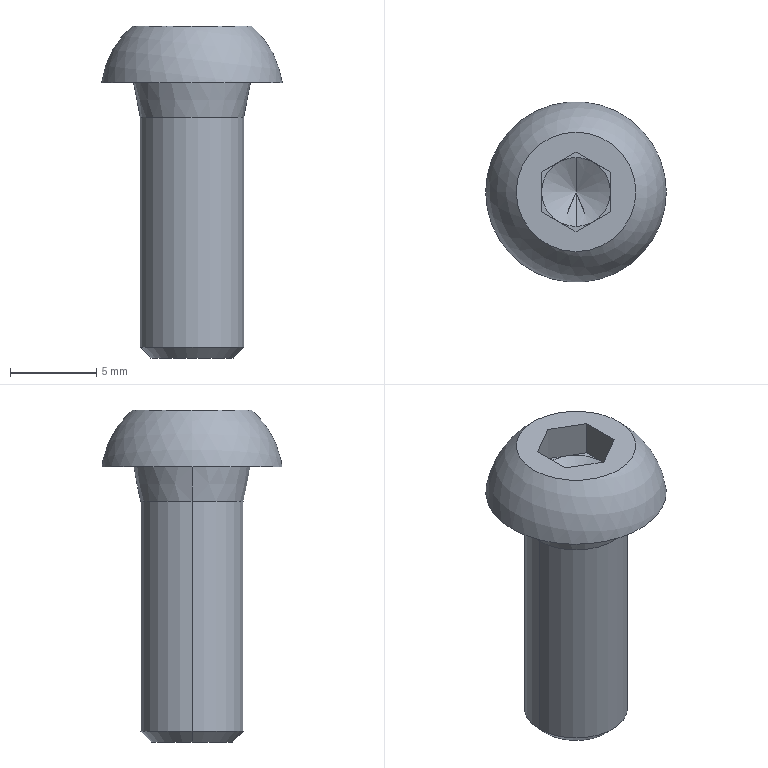Part | SolidWorks | features BaseBody 1 | 1 solid | 24 faces | box 10.5 x 10.5 x 19.3 mm | volume 647.467 mm3 | plane 15 | cone 6 | cylinder 2 | sphere 1 | commonest cylinder face diameters 6 x2
STEP:
#1=CARTESIAN_POINT('',(3.,0.,-13.387));
#2=VERTEX_POINT('',#1);
#3=CARTESIAN_POINT('',(-3.,0.,-13.387));
#4=VERTEX_POINT('',#3);
#5=CARTESIAN_POINT('',(0.,0.,-13.387));
#6=DIRECTION('',(0.,0.,1.));
#7=DIRECTION('',(1.,0.,0.));
#8=AXIS2_PLACEMENT_3D('',#5,#6,#7);
#9=CIRCLE('',#8,3.);
#10=EDGE_CURVE('',#2,#4,#9,.T.);
#11=ORIENTED_EDGE('',*,*,#10,.T.);
#12=CARTESIAN_POINT('',(-3.,0.,0.));
#13=VERTEX_POINT('',#12);
#14=CARTESIAN_POINT('',(-3.,0.,-14.));
#15=DIRECTION('',(0.,0.,1.));
#16=VECTOR('',#15,1000.);
#17=LINE('',#14,#16);
#18=EDGE_CURVE('',#4,#13,#17,.T.);
#19=ORIENTED_EDGE('',*,*,#18,.T.);
#20=CARTESIAN_POINT('',(3.,0.,0.));
#21=VERTEX_POINT('',#20);
#22=CARTESIAN_POINT('',(0.,0.,0.));
#23=DIRECTION('',(0.,0.,-1.));
#24=DIRECTION('',(1.,0.,0.));
#25=AXIS2_PLACEMENT_3D('',#22,#23,#24);
#26=CIRCLE('',#25,3.);
#27=EDGE_CURVE('',#13,#21,#26,.T.);
#28=ORIENTED_EDGE('',*,*,#27,.T.);
#29=CARTESIAN_POINT('',(3.,0.,-14.));
#30=DIRECTION('',(0.,0.,1.));
#31=VECTOR('',#30,1000.);
#32=LINE('',#29,#31);
#33=EDGE_CURVE('',#2,#21,#32,.T.);
#34=ORIENTED_EDGE('',*,*,#33,.F.);
#35=EDGE_LOOP('',(#11,#19,#28,#34));
#36=FACE_OUTER_BOUND('',#35,.T.);
#37=CARTESIAN_POINT('',(0.,0.,-14.));
#38=DIRECTION('',(0.,0.,1.));
#39=DIRECTION('',(1.,0.,0.));
#40=AXIS2_PLACEMENT_3D('',#37,#38,#39);
#41=CYLINDRICAL_SURFACE('',#40,3.);
#42=ADVANCED_FACE('',(#36),#41,.T.);
#43=ORIENTED_EDGE('',*,*,#27,.F.);
#44=CARTESIAN_POINT('',(-3.4,0.,2.));
#45=VERTEX_POINT('',#44);
#46=CARTESIAN_POINT('',(-3.4,0.,2.));
#47=DIRECTION('',(-0.1961,0.,0.9806));
#48=VECTOR('',#47,1000.);
#49=LINE('',#46,#48);
#50=EDGE_CURVE('',#13,#45,#49,.T.);
#51=ORIENTED_EDGE('',*,*,#50,.T.);
#52=CARTESIAN_POINT('',(3.4,0.,2.));
#53=VERTEX_POINT('',#52);
#54=CARTESIAN_POINT('',(0.,0.,2.));
#55=DIRECTION('',(0.,0.,-1.));
#56=DIRECTION('',(1.,0.,0.));
#57=AXIS2_PLACEMENT_3D('',#54,#55,#56);
#58=CIRCLE('',#57,3.4);
#59=EDGE_CURVE('',#45,#53,#58,.T.);
#60=ORIENTED_EDGE('',*,*,#59,.T.);
#61=CARTESIAN_POINT('',(3.4,0.,2.));
#62=DIRECTION('',(0.1961,0.,0.9806));
#63=VECTOR('',#62,1000.);
#64=LINE('',#61,#63);
#65=EDGE_CURVE('',#21,#53,#64,.T.);
#66=ORIENTED_EDGE('',*,*,#65,.F.);
#67=EDGE_LOOP('',(#43,#51,#60,#66));
#68=FACE_OUTER_BOUND('',#67,.T.);
#69=CARTESIAN_POINT('',(0.,0.,2.));
#70=DIRECTION('',(0.,0.,1.));
#71=DIRECTION('',(1.,0.,0.));
#72=AXIS2_PLACEMENT_3D('',#69,#70,#71);
#73=CONICAL_SURFACE('',#72,3.4,0.1974);
#74=ADVANCED_FACE('',(#68),#73,.T.);
#75=CARTESIAN_POINT('',(2.386,0.,-14.));
#76=VERTEX_POINT('',#75);
#77=CARTESIAN_POINT('',(-2.386,0.,-14.));
#78=VERTEX_POINT('',#77);
#79=CARTESIAN_POINT('',(0.,0.,-14.));
#80=DIRECTION('',(0.,0.,1.));
#81=DIRECTION('',(1.,0.,0.));
#82=AXIS2_PLACEMENT_3D('',#79,#80,#81);
#83=CIRCLE('',#82,2.386);
#84=EDGE_CURVE('',#76,#78,#83,.T.);
#85=ORIENTED_EDGE('',*,*,#84,.T.);
#86=CARTESIAN_POINT('',(-3.,0.,-13.387));
#87=DIRECTION('',(-0.7071,0.,0.7071));
#88=VECTOR('',#87,1000.);
#89=LINE('',#86,#88);
#90=EDGE_CURVE('',#78,#4,#89,.T.);
#91=ORIENTED_EDGE('',*,*,#90,.T.);
#92=ORIENTED_EDGE('',*,*,#10,.F.);
#93=CARTESIAN_POINT('',(3.,0.,-13.387));
#94=DIRECTION('',(0.7071,0.,0.7071));
#95=VECTOR('',#94,1000.);
#96=LINE('',#93,#95);
#97=EDGE_CURVE('',#76,#2,#96,.T.);
#98=ORIENTED_EDGE('',*,*,#97,.F.);
#99=EDGE_LOOP('',(#85,#91,#92,#98));
#100=FACE_OUTER_BOUND('',#99,.T.);
#101=CARTESIAN_POINT('',(0.,0.,-13.387));
#102=DIRECTION('',(0.,0.,1.));
#103=DIRECTION('',(1.,0.,0.));
#104=AXIS2_PLACEMENT_3D('',#101,#102,#103);
#105=CONICAL_SURFACE('',#104,3.,0.7854);
#106=ADVANCED_FACE('',(#100),#105,.T.);
#107=CARTESIAN_POINT('',(0.,0.,2.065));
#108=VERTEX_POINT('',#107);
#109=CARTESIAN_POINT('',(0.,-2.,3.22));
#110=VERTEX_POINT('',#109);
#111=CARTESIAN_POINT('',(0.,-2.,3.22));
#112=DIRECTION('',(0.,-0.866,0.5));
#113=VECTOR('',#112,1000.);
#114=LINE('',#111,#113);
#115=EDGE_CURVE('',#108,#110,#114,.T.);
#116=ORIENTED_EDGE('',*,*,#115,.F.);
#117=CARTESIAN_POINT('',(0.,2.,3.22));
#118=VERTEX_POINT('',#117);
#119=CARTESIAN_POINT('',(0.,2.,3.22));
#120=DIRECTION('',(0.,0.866,0.5));
#121=VECTOR('',#120,1000.);
#122=LINE('',#119,#121);
#123=EDGE_CURVE('',#108,#118,#122,.T.);
#124=ORIENTED_EDGE('',*,*,#123,.T.);
#125=CARTESIAN_POINT('',(-1.,1.732,3.22));
#126=VERTEX_POINT('',#125);
#127=CARTESIAN_POINT('',(0.,0.,3.22));
#128=DIRECTION('',(0.,0.,-1.));
#129=DIRECTION('',(0.,-1.,0.));
#130=AXIS2_PLACEMENT_3D('',#127,#128,#129);
#131=CIRCLE('',#130,2.);
#132=EDGE_CURVE('',#126,#118,#131,.T.);
#133=ORIENTED_EDGE('',*,*,#132,.F.);
#134=CARTESIAN_POINT('',(-2.,0.,3.22));
#135=VERTEX_POINT('',#134);
#136=CARTESIAN_POINT('',(0.,0.,3.22));
#137=DIRECTION('',(0.,0.,-1.));
#138=DIRECTION('',(0.,-1.,0.));
#139=AXIS2_PLACEMENT_3D('',#136,#137,#138);
#140=CIRCLE('',#139,2.);
#141=EDGE_CURVE('',#135,#126,#140,.T.);
#142=ORIENTED_EDGE('',*,*,#141,.F.);
#143=CARTESIAN_POINT('',(-1.,-1.732,3.22));
#144=VERTEX_POINT('',#143);
#145=CARTESIAN_POINT('',(0.,0.,3.22));
#146=DIRECTION('',(0.,0.,-1.));
#147=DIRECTION('',(0.,-1.,0.));
#148=AXIS2_PLACEMENT_3D('',#145,#146,#147);
#149=CIRCLE('',#148,2.);
#150=EDGE_CURVE('',#144,#135,#149,.T.);
#151=ORIENTED_EDGE('',*,*,#150,.F.);
#152=CARTESIAN_POINT('',(0.,0.,3.22));
#153=DIRECTION('',(0.,0.,-1.));
#154=DIRECTION('',(0.,-1.,0.));
#155=AXIS2_PLACEMENT_3D('',#152,#153,#154);
#156=CIRCLE('',#155,2.);
#157=EDGE_CURVE('',#110,#144,#156,.T.);
#158=ORIENTED_EDGE('',*,*,#157,.F.);
#159=EDGE_LOOP('',(#116,#124,#133,#142,#151,#158));
#160=FACE_OUTER_BOUND('',#159,.T.);
#161=CARTESIAN_POINT('',(0.,0.,3.22));
#162=DIRECTION('',(0.,0.,1.));
#163=DIRECTION('',(0.,-1.,0.));
#164=AXIS2_PLACEMENT_3D('',#161,#162,#163);
#165=CONICAL_SURFACE('',#164,2.,1.047);
#166=ADVANCED_FACE('',(#160),#165,.F.);
#167=ORIENTED_EDGE('',*,*,#18,.F.);
#168=CARTESIAN_POINT('',(0.,0.,-13.387));
#169=DIRECTION('',(0.,0.,1.));
#170=DIRECTION('',(1.,0.,0.));
#171=AXIS2_PLACEMENT_3D('',#168,#169,#170);
#172=CIRCLE('',#171,3.);
#173=EDGE_CURVE('',#4,#2,#172,.T.);
#174=ORIENTED_EDGE('',*,*,#173,.T.);
#175=ORIENTED_EDGE('',*,*,#33,.T.);
#176=CARTESIAN_POINT('',(0.,0.,0.));
#177=DIRECTION('',(0.,0.,-1.));
#178=DIRECTION('',(1.,0.,0.));
#179=AXIS2_PLACEMENT_3D('',#176,#177,#178);
#180=CIRCLE('',#179,3.);
#181=EDGE_CURVE('',#21,#13,#180,.T.);
#182=ORIENTED_EDGE('',*,*,#181,.T.);
#183=EDGE_LOOP('',(#167,#174,#175,#182));
#184=FACE_OUTER_BOUND('',#183,.T.);
#185=CARTESIAN_POINT('',(0.,0.,-14.));
#186=DIRECTION('',(0.,0.,1.));
#187=DIRECTION('',(1.,0.,0.));
#188=AXIS2_PLACEMENT_3D('',#185,#186,#187);
#189=CYLINDRICAL_SURFACE('',#188,3.);
#190=ADVANCED_FACE('',(#184),#189,.T.);
#191=ORIENTED_EDGE('',*,*,#50,.F.);
#192=ORIENTED_EDGE('',*,*,#181,.F.);
#193=ORIENTED_EDGE('',*,*,#65,.T.);
#194=CARTESIAN_POINT('',(0.,0.,2.));
#195=DIRECTION('',(0.,0.,-1.));
#196=DIRECTION('',(1.,0.,0.));
#197=AXIS2_PLACEMENT_3D('',#194,#195,#196);
#198=CIRCLE('',#197,3.4);
#199=EDGE_CURVE('',#53,#45,#198,.T.);
#200=ORIENTED_EDGE('',*,*,#199,.T.);
#201=EDGE_LOOP('',(#191,#192,#193,#200));
#202=FACE_OUTER_BOUND('',#201,.T.);
#203=CARTESIAN_POINT('',(0.,0.,2.));
#204=DIRECTION('',(0.,0.,1.));
#205=DIRECTION('',(1.,0.,0.));
#206=AXIS2_PLACEMENT_3D('',#203,#204,#205);
#207=CONICAL_SURFACE('',#206,3.4,0.1974);
#208=ADVANCED_FACE('',(#202),#207,.T.);
#209=ORIENTED_EDGE('',*,*,#90,.F.);
#210=CARTESIAN_POINT('',(0.,0.,-14.));
#211=DIRECTION('',(0.,0.,1.));
#212=DIRECTION('',(1.,0.,0.));
#213=AXIS2_PLACEMENT_3D('',#210,#211,#212);
#214=CIRCLE('',#213,2.386);
#215=EDGE_CURVE('',#78,#76,#214,.T.);
#216=ORIENTED_EDGE('',*,*,#215,.T.);
#217=ORIENTED_EDGE('',*,*,#97,.T.);
#218=ORIENTED_EDGE('',*,*,#173,.F.);
#219=EDGE_LOOP('',(#209,#216,#217,#218));
#220=FACE_OUTER_BOUND('',#219,.T.);
#221=CARTESIAN_POINT('',(0.,0.,-13.387));
#222=DIRECTION('',(0.,0.,1.));
#223=DIRECTION('',(1.,0.,0.));
#224=AXIS2_PLACEMENT_3D('',#221,#222,#223);
#225=CONICAL_SURFACE('',#224,3.,0.7854);
#226=ADVANCED_FACE('',(#220),#225,.T.);
#227=ORIENTED_EDGE('',*,*,#199,.F.);
#228=ORIENTED_EDGE('',*,*,#59,.F.);
#229=EDGE_LOOP('',(#227,#228));
#230=FACE_BOUND('',#229,.T.);
#231=CARTESIAN_POINT('',(5.25,0.,2.));
#232=VERTEX_POINT('',#231);
#233=CARTESIAN_POINT('',(-5.25,0.,2.));
#234=VERTEX_POINT('',#233);
#235=CARTESIAN_POINT('',(0.,0.,2.));
#236=DIRECTION('',(0.,0.,1.));
#237=DIRECTION('',(1.,0.,0.));
#238=AXIS2_PLACEMENT_3D('',#235,#236,#237);
#239=CIRCLE('',#238,5.25);
#240=EDGE_CURVE('',#232,#234,#239,.T.);
#241=ORIENTED_EDGE('',*,*,#240,.F.);
#242=CARTESIAN_POINT('',(0.,0.,2.));
#243=DIRECTION('',(0.,0.,1.));
#244=DIRECTION('',(1.,0.,0.));
#245=AXIS2_PLACEMENT_3D('',#242,#243,#244);
#246=CIRCLE('',#245,5.25);
#247=EDGE_CURVE('',#234,#232,#246,.T.);
#248=ORIENTED_EDGE('',*,*,#247,.F.);
#249=EDGE_LOOP('',(#241,#248));
#250=FACE_OUTER_BOUND('',#249,.T.);
#251=CARTESIAN_POINT('',(0.,5.25,2.));
#252=DIRECTION('',(0.,0.,1.));
#253=DIRECTION('',(1.,0.,0.));
#254=AXIS2_PLACEMENT_3D('',#251,#252,#253);
#255=PLANE('',#254);
#256=ADVANCED_FACE('',(#230,#250),#255,.F.);
#257=ORIENTED_EDGE('',*,*,#84,.F.);
#258=ORIENTED_EDGE('',*,*,#215,.F.);
#259=EDGE_LOOP('',(#257,#258));
#260=FACE_OUTER_BOUND('',#259,.T.);
#261=CARTESIAN_POINT('',(0.,2.386,-14.));
#262=DIRECTION('',(0.,0.,1.));
#263=DIRECTION('',(1.,0.,0.));
#264=AXIS2_PLACEMENT_3D('',#261,#262,#263);
#265=PLANE('',#264);
#266=ADVANCED_FACE('',(#260),#265,.F.);
#267=CARTESIAN_POINT('',(-3.472,0.,5.3));
#268=VERTEX_POINT('',#267);
#269=CARTESIAN_POINT('',(3.472,0.,5.3));
#270=VERTEX_POINT('',#269);
#271=CARTESIAN_POINT('',(0.,0.,5.3));
#272=DIRECTION('',(0.,0.,-1.));
#273=DIRECTION('',(-1.,0.,0.));
#274=AXIS2_PLACEMENT_3D('',#271,#272,#273);
#275=CIRCLE('',#274,3.472);
#276=EDGE_CURVE('',#268,#270,#275,.T.);
#277=ORIENTED_EDGE('',*,*,#276,.T.);
#278=CARTESIAN_POINT('',(0.,0.,5.3));
#279=DIRECTION('',(0.,0.,-1.));
#280=DIRECTION('',(-1.,0.,0.));
#281=AXIS2_PLACEMENT_3D('',#278,#279,#280);
#282=CIRCLE('',#281,3.472);
#283=EDGE_CURVE('',#270,#268,#282,.T.);
#284=ORIENTED_EDGE('',*,*,#283,.T.);
#285=EDGE_LOOP('',(#277,#284));
#286=FACE_BOUND('',#285,.T.);
#287=ORIENTED_EDGE('',*,*,#240,.T.);
#288=ORIENTED_EDGE('',*,*,#247,.T.);
#289=EDGE_LOOP('',(#287,#288));
#290=FACE_OUTER_BOUND('',#289,.T.);
#291=CARTESIAN_POINT('',(0.,0.,1.3));
#292=DIRECTION('',(0.115,0.,0.9934));
#293=DIRECTION('',(-0.9934,0.,0.115));
#294=AXIS2_PLACEMENT_3D('',#291,#292,#293);
#295=SPHERICAL_SURFACE('',#294,5.296);
#296=ADVANCED_FACE('',(#286,#290),#295,.T.);
#297=ORIENTED_EDGE('',*,*,#276,.F.);
#298=ORIENTED_EDGE('',*,*,#283,.F.);
#299=EDGE_LOOP('',(#297,#298));
#300=FACE_OUTER_BOUND('',#299,.T.);
#301=CARTESIAN_POINT('',(-2.,1.155,5.3));
#302=VERTEX_POINT('',#301);
#303=CARTESIAN_POINT('',(-2.,-1.155,5.3));
#304=VERTEX_POINT('',#303);
#305=CARTESIAN_POINT('',(-2.,0.,5.3));
#306=DIRECTION('',(0.,-1.,0.));
#307=VECTOR('',#306,1000.);
#308=LINE('',#305,#307);
#309=EDGE_CURVE('',#302,#304,#308,.T.);
#310=ORIENTED_EDGE('',*,*,#309,.F.);
#311=CARTESIAN_POINT('',(0.,2.309,5.3));
#312=VERTEX_POINT('',#311);
#313=CARTESIAN_POINT('',(0.,2.309,5.3));
#314=DIRECTION('',(-0.866,-0.5,0.));
#315=VECTOR('',#314,1000.);
#316=LINE('',#313,#315);
#317=EDGE_CURVE('',#312,#302,#316,.T.);
#318=ORIENTED_EDGE('',*,*,#317,.F.);
#319=CARTESIAN_POINT('',(2.,1.155,5.3));
#320=VERTEX_POINT('',#319);
#321=CARTESIAN_POINT('',(2.,1.155,5.3));
#322=DIRECTION('',(-0.866,0.5,0.));
#323=VECTOR('',#322,1000.);
#324=LINE('',#321,#323);
#325=EDGE_CURVE('',#320,#312,#324,.T.);
#326=ORIENTED_EDGE('',*,*,#325,.F.);
#327=CARTESIAN_POINT('',(2.,-1.155,5.3));
#328=VERTEX_POINT('',#327);
#329=CARTESIAN_POINT('',(2.,0.,5.3));
#330=DIRECTION('',(0.,1.,0.));
#331=VECTOR('',#330,1000.);
#332=LINE('',#329,#331);
#333=EDGE_CURVE('',#328,#320,#332,.T.);
#334=ORIENTED_EDGE('',*,*,#333,.F.);
#335=CARTESIAN_POINT('',(0.,-2.309,5.3));
#336=VERTEX_POINT('',#335);
#337=CARTESIAN_POINT('',(0.,-2.309,5.3));
#338=DIRECTION('',(0.866,0.5,0.));
#339=VECTOR('',#338,1000.);
#340=LINE('',#337,#339);
#341=EDGE_CURVE('',#336,#328,#340,.T.);
#342=ORIENTED_EDGE('',*,*,#341,.F.);
#343=CARTESIAN_POINT('',(-2.,-1.155,5.3));
#344=DIRECTION('',(0.866,-0.5,0.));
#345=VECTOR('',#344,1000.);
#346=LINE('',#343,#345);
#347=EDGE_CURVE('',#304,#336,#346,.T.);
#348=ORIENTED_EDGE('',*,*,#347,.F.);
#349=EDGE_LOOP('',(#310,#318,#326,#334,#342,#348));
#350=FACE_BOUND('',#349,.T.);
#351=CARTESIAN_POINT('',(0.,0.,5.3));
#352=DIRECTION('',(0.,0.,-1.));
#353=DIRECTION('',(-1.,0.,0.));
#354=AXIS2_PLACEMENT_3D('',#351,#352,#353);
#355=PLANE('',#354);
#356=ADVANCED_FACE('',(#300,#350),#355,.F.);
#357=CARTESIAN_POINT('',(0.,-2.309,3.22));
#358=VERTEX_POINT('',#357);
#359=CARTESIAN_POINT('',(-2.,-1.155,3.22));
#360=DIRECTION('',(0.866,-0.5,0.));
#361=VECTOR('',#360,1000.);
#362=LINE('',#359,#361);
#363=EDGE_CURVE('',#144,#358,#362,.T.);
#364=ORIENTED_EDGE('',*,*,#363,.F.);
#365=CARTESIAN_POINT('',(-2.,-1.155,3.22));
#366=VERTEX_POINT('',#365);
#367=CARTESIAN_POINT('',(-2.,-1.155,3.22));
#368=DIRECTION('',(0.866,-0.5,0.));
#369=VECTOR('',#368,1000.);
#370=LINE('',#367,#369);
#371=EDGE_CURVE('',#366,#144,#370,.T.);
#372=ORIENTED_EDGE('',*,*,#371,.F.);
#373=CARTESIAN_POINT('',(-2.,-1.155,3.22));
#374=DIRECTION('',(0.,0.,-1.));
#375=VECTOR('',#374,1000.);
#376=LINE('',#373,#375);
#377=EDGE_CURVE('',#304,#366,#376,.T.);
#378=ORIENTED_EDGE('',*,*,#377,.F.);
#379=ORIENTED_EDGE('',*,*,#347,.T.);
#380=CARTESIAN_POINT('',(0.,-2.309,3.22));
#381=DIRECTION('',(0.,0.,1.));
#382=VECTOR('',#381,1000.);
#383=LINE('',#380,#382);
#384=EDGE_CURVE('',#358,#336,#383,.T.);
#385=ORIENTED_EDGE('',*,*,#384,.F.);
#386=EDGE_LOOP('',(#364,#372,#378,#379,#385));
#387=FACE_OUTER_BOUND('',#386,.T.);
#388=CARTESIAN_POINT('',(-2.,-1.155,3.22));
#389=DIRECTION('',(-0.5,-0.866,0.));
#390=DIRECTION('',(0.866,-0.5,0.));
#391=AXIS2_PLACEMENT_3D('',#388,#389,#390);
#392=PLANE('',#391);
#393=ADVANCED_FACE('',(#387),#392,.F.);
#394=CARTESIAN_POINT('',(-2.,0.,3.22));
#395=DIRECTION('',(0.,-1.,0.));
#396=VECTOR('',#395,1000.);
#397=LINE('',#394,#396);
#398=EDGE_CURVE('',#135,#366,#397,.T.);
#399=ORIENTED_EDGE('',*,*,#398,.F.);
#400=CARTESIAN_POINT('',(-2.,1.155,3.22));
#401=VERTEX_POINT('',#400);
#402=CARTESIAN_POINT('',(-2.,0.,3.22));
#403=DIRECTION('',(0.,-1.,0.));
#404=VECTOR('',#403,1000.);
#405=LINE('',#402,#404);
#406=EDGE_CURVE('',#401,#135,#405,.T.);
#407=ORIENTED_EDGE('',*,*,#406,.F.);
#408=CARTESIAN_POINT('',(-2.,1.155,3.22));
#409=DIRECTION('',(0.,0.,-1.));
#410=VECTOR('',#409,1000.);
#411=LINE('',#408,#410);
#412=EDGE_CURVE('',#302,#401,#411,.T.);
#413=ORIENTED_EDGE('',*,*,#412,.F.);
#414=ORIENTED_EDGE('',*,*,#309,.T.);
#415=ORIENTED_EDGE('',*,*,#377,.T.);
#416=EDGE_LOOP('',(#399,#407,#413,#414,#415));
#417=FACE_OUTER_BOUND('',#416,.T.);
#418=CARTESIAN_POINT('',(-2.,1.155,3.22));
#419=DIRECTION('',(-1.,0.,0.));
#420=DIRECTION('',(0.,0.,1.));
#421=AXIS2_PLACEMENT_3D('',#418,#419,#420);
#422=PLANE('',#421);
#423=ADVANCED_FACE('',(#417),#422,.F.);
#424=CARTESIAN_POINT('',(-1.,1.732,3.22));
#425=DIRECTION('',(-0.866,-0.5,0.));
#426=VECTOR('',#425,1000.);
#427=LINE('',#424,#426);
#428=EDGE_CURVE('',#126,#401,#427,.T.);
#429=ORIENTED_EDGE('',*,*,#428,.F.);
#430=CARTESIAN_POINT('',(0.,2.309,3.22));
#431=VERTEX_POINT('',#430);
#432=CARTESIAN_POINT('',(0.,2.309,3.22));
#433=DIRECTION('',(-0.866,-0.5,0.));
#434=VECTOR('',#433,1000.);
#435=LINE('',#432,#434);
#436=EDGE_CURVE('',#431,#126,#435,.T.);
#437=ORIENTED_EDGE('',*,*,#436,.F.);
#438=CARTESIAN_POINT('',(0.,2.309,3.22));
#439=DIRECTION('',(0.,0.,-1.));
#440=VECTOR('',#439,1000.);
#441=LINE('',#438,#440);
#442=EDGE_CURVE('',#312,#431,#441,.T.);
#443=ORIENTED_EDGE('',*,*,#442,.F.);
#444=ORIENTED_EDGE('',*,*,#317,.T.);
#445=ORIENTED_EDGE('',*,*,#412,.T.);
#446=EDGE_LOOP('',(#429,#437,#443,#444,#445));
#447=FACE_OUTER_BOUND('',#446,.T.);
#448=CARTESIAN_POINT('',(0.,2.309,3.22));
#449=DIRECTION('',(-0.5,0.866,0.));
#450=DIRECTION('',(-0.866,-0.5,0.));
#451=AXIS2_PLACEMENT_3D('',#448,#449,#450);
#452=PLANE('',#451);
#453=ADVANCED_FACE('',(#447),#452,.F.);
#454=CARTESIAN_POINT('',(1.,1.732,3.22));
#455=VERTEX_POINT('',#454);
#456=CARTESIAN_POINT('',(2.,1.155,3.22));
#457=DIRECTION('',(-0.866,0.5,0.));
#458=VECTOR('',#457,1000.);
#459=LINE('',#456,#458);
#460=EDGE_CURVE('',#455,#431,#459,.T.);
#461=ORIENTED_EDGE('',*,*,#460,.F.);
#462=CARTESIAN_POINT('',(2.,1.155,3.22));
#463=VERTEX_POINT('',#462);
#464=CARTESIAN_POINT('',(2.,1.155,3.22));
#465=DIRECTION('',(-0.866,0.5,0.));
#466=VECTOR('',#465,1000.);
#467=LINE('',#464,#466);
#468=EDGE_CURVE('',#463,#455,#467,.T.);
#469=ORIENTED_EDGE('',*,*,#468,.F.);
#470=CARTESIAN_POINT('',(2.,1.155,3.22));
#471=DIRECTION('',(0.,0.,-1.));
#472=VECTOR('',#471,1000.);
#473=LINE('',#470,#472);
#474=EDGE_CURVE('',#320,#463,#473,.T.);
#475=ORIENTED_EDGE('',*,*,#474,.F.);
#476=ORIENTED_EDGE('',*,*,#325,.T.);
#477=ORIENTED_EDGE('',*,*,#442,.T.);
#478=EDGE_LOOP('',(#461,#469,#475,#476,#477));
#479=FACE_OUTER_BOUND('',#478,.T.);
#480=CARTESIAN_POINT('',(2.,1.155,3.22));
#481=DIRECTION('',(0.5,0.866,0.));
#482=DIRECTION('',(-0.866,0.5,0.));
#483=AXIS2_PLACEMENT_3D('',#480,#481,#482);
#484=PLANE('',#483);
#485=ADVANCED_FACE('',(#479),#484,.F.);
#486=CARTESIAN_POINT('',(2.,0.,3.22));
#487=VERTEX_POINT('',#486);
#488=CARTESIAN_POINT('',(2.,0.,3.22));
#489=DIRECTION('',(0.,1.,0.));
#490=VECTOR('',#489,1000.);
#491=LINE('',#488,#490);
#492=EDGE_CURVE('',#487,#463,#491,.T.);
#493=ORIENTED_EDGE('',*,*,#492,.F.);
#494=CARTESIAN_POINT('',(2.,-1.155,3.22));
#495=VERTEX_POINT('',#494);
#496=CARTESIAN_POINT('',(2.,0.,3.22));
#497=DIRECTION('',(0.,1.,0.));
#498=VECTOR('',#497,1000.);
#499=LINE('',#496,#498);
#500=EDGE_CURVE('',#495,#487,#499,.T.);
#501=ORIENTED_EDGE('',*,*,#500,.F.);
#502=CARTESIAN_POINT('',(2.,-1.155,3.22));
#503=DIRECTION('',(0.,0.,-1.));
#504=VECTOR('',#503,1000.);
#505=LINE('',#502,#504);
#506=EDGE_CURVE('',#328,#495,#505,.T.);
#507=ORIENTED_EDGE('',*,*,#506,.F.);
#508=ORIENTED_EDGE('',*,*,#333,.T.);
#509=ORIENTED_EDGE('',*,*,#474,.T.);
#510=EDGE_LOOP('',(#493,#501,#507,#508,#509));
#511=FACE_OUTER_BOUND('',#510,.T.);
#512=CARTESIAN_POINT('',(2.,-1.155,3.22));
#513=DIRECTION('',(1.,0.,0.));
#514=DIRECTION('',(0.,0.,-1.));
#515=AXIS2_PLACEMENT_3D('',#512,#513,#514);
#516=PLANE('',#515);
#517=ADVANCED_FACE('',(#511),#516,.F.);
#518=CARTESIAN_POINT('',(1.,-1.732,3.22));
#519=VERTEX_POINT('',#518);
#520=CARTESIAN_POINT('',(0.,-2.309,3.22));
#521=DIRECTION('',(0.866,0.5,0.));
#522=VECTOR('',#521,1000.);
#523=LINE('',#520,#522);
#524=EDGE_CURVE('',#519,#495,#523,.T.);
#525=ORIENTED_EDGE('',*,*,#524,.F.);
#526=CARTESIAN_POINT('',(0.,-2.309,3.22));
#527=DIRECTION('',(0.866,0.5,0.));
#528=VECTOR('',#527,1000.);
#529=LINE('',#526,#528);
#530=EDGE_CURVE('',#358,#519,#529,.T.);
#531=ORIENTED_EDGE('',*,*,#530,.F.);
#532=ORIENTED_EDGE('',*,*,#384,.T.);
#533=ORIENTED_EDGE('',*,*,#341,.T.);
#534=ORIENTED_EDGE('',*,*,#506,.T.);
#535=EDGE_LOOP('',(#525,#531,#532,#533,#534));
#536=FACE_OUTER_BOUND('',#535,.T.);
#537=CARTESIAN_POINT('',(0.,-2.309,3.22));
#538=DIRECTION('',(0.5,-0.866,0.));
#539=DIRECTION('',(0.866,0.5,0.));
#540=AXIS2_PLACEMENT_3D('',#537,#538,#539);
#541=PLANE('',#540);
#542=ADVANCED_FACE('',(#536),#541,.F.);
#543=ORIENTED_EDGE('',*,*,#363,.T.);
#544=ORIENTED_EDGE('',*,*,#530,.T.);
#545=CARTESIAN_POINT('',(0.,0.,3.22));
#546=DIRECTION('',(0.,0.,-1.));
#547=DIRECTION('',(0.,-1.,0.));
#548=AXIS2_PLACEMENT_3D('',#545,#546,#547);
#549=CIRCLE('',#548,2.);
#550=EDGE_CURVE('',#519,#110,#549,.T.);
#551=ORIENTED_EDGE('',*,*,#550,.T.);
#552=ORIENTED_EDGE('',*,*,#157,.T.);
#553=EDGE_LOOP('',(#543,#544,#551,#552));
#554=FACE_OUTER_BOUND('',#553,.T.);
#555=CARTESIAN_POINT('',(0.,0.,3.22));
#556=DIRECTION('',(0.,0.,1.));
#557=DIRECTION('',(1.,0.,0.));
#558=AXIS2_PLACEMENT_3D('',#555,#556,#557);
#559=PLANE('',#558);
#560=ADVANCED_FACE('',(#554),#559,.T.);
#561=ORIENTED_EDGE('',*,*,#460,.T.);
#562=ORIENTED_EDGE('',*,*,#436,.T.);
#563=ORIENTED_EDGE('',*,*,#132,.T.);
#564=CARTESIAN_POINT('',(0.,0.,3.22));
#565=DIRECTION('',(0.,0.,-1.));
#566=DIRECTION('',(0.,-1.,0.));
#567=AXIS2_PLACEMENT_3D('',#564,#565,#566);
#568=CIRCLE('',#567,2.);
#569=EDGE_CURVE('',#118,#455,#568,.T.);
#570=ORIENTED_EDGE('',*,*,#569,.T.);
#571=EDGE_LOOP('',(#561,#562,#563,#570));
#572=FACE_OUTER_BOUND('',#571,.T.);
#573=CARTESIAN_POINT('',(0.,0.,3.22));
#574=DIRECTION('',(0.,0.,1.));
#575=DIRECTION('',(1.,0.,0.));
#576=AXIS2_PLACEMENT_3D('',#573,#574,#575);
#577=PLANE('',#576);
#578=ADVANCED_FACE('',(#572),#577,.T.);
#579=ORIENTED_EDGE('',*,*,#524,.T.);
#580=ORIENTED_EDGE('',*,*,#500,.T.);
#581=CARTESIAN_POINT('',(0.,0.,3.22));
#582=DIRECTION('',(0.,0.,-1.));
#583=DIRECTION('',(0.,-1.,0.));
#584=AXIS2_PLACEMENT_3D('',#581,#582,#583);
#585=CIRCLE('',#584,2.);
#586=EDGE_CURVE('',#487,#519,#585,.T.);
#587=ORIENTED_EDGE('',*,*,#586,.T.);
#588=EDGE_LOOP('',(#579,#580,#587));
#589=FACE_OUTER_BOUND('',#588,.T.);
#590=CARTESIAN_POINT('',(0.,0.,3.22));
#591=DIRECTION('',(0.,0.,1.));
#592=DIRECTION('',(1.,0.,0.));
#593=AXIS2_PLACEMENT_3D('',#590,#591,#592);
#594=PLANE('',#593);
#595=ADVANCED_FACE('',(#589),#594,.T.);
#596=ORIENTED_EDGE('',*,*,#123,.F.);
#597=ORIENTED_EDGE('',*,*,#115,.T.);
#598=ORIENTED_EDGE('',*,*,#550,.F.);
#599=ORIENTED_EDGE('',*,*,#586,.F.);
#600=CARTESIAN_POINT('',(0.,0.,3.22));
#601=DIRECTION('',(0.,0.,-1.));
#602=DIRECTION('',(0.,-1.,0.));
#603=AXIS2_PLACEMENT_3D('',#600,#601,#602);
#604=CIRCLE('',#603,2.);
#605=EDGE_CURVE('',#455,#487,#604,.T.);
#606=ORIENTED_EDGE('',*,*,#605,.F.);
#607=ORIENTED_EDGE('',*,*,#569,.F.);
#608=EDGE_LOOP('',(#596,#597,#598,#599,#606,#607));
#609=FACE_OUTER_BOUND('',#608,.T.);
#610=CARTESIAN_POINT('',(0.,0.,3.22));
#611=DIRECTION('',(0.,0.,1.));
#612=DIRECTION('',(0.,-1.,0.));
#613=AXIS2_PLACEMENT_3D('',#610,#611,#612);
#614=CONICAL_SURFACE('',#613,2.,1.047);
#615=ADVANCED_FACE('',(#609),#614,.F.);
#616=ORIENTED_EDGE('',*,*,#492,.T.);
#617=ORIENTED_EDGE('',*,*,#468,.T.);
#618=ORIENTED_EDGE('',*,*,#605,.T.);
#619=EDGE_LOOP('',(#616,#617,#618));
#620=FACE_OUTER_BOUND('',#619,.T.);
#621=CARTESIAN_POINT('',(0.,0.,3.22));
#622=DIRECTION('',(0.,0.,1.));
#623=DIRECTION('',(1.,0.,0.));
#624=AXIS2_PLACEMENT_3D('',#621,#622,#623);
#625=PLANE('',#624);
#626=ADVANCED_FACE('',(#620),#625,.T.);
#627=ORIENTED_EDGE('',*,*,#428,.T.);
#628=ORIENTED_EDGE('',*,*,#406,.T.);
#629=ORIENTED_EDGE('',*,*,#141,.T.);
#630=EDGE_LOOP('',(#627,#628,#629));
#631=FACE_OUTER_BOUND('',#630,.T.);
#632=CARTESIAN_POINT('',(0.,0.,3.22));
#633=DIRECTION('',(0.,0.,1.));
#634=DIRECTION('',(1.,0.,0.));
#635=AXIS2_PLACEMENT_3D('',#632,#633,#634);
#636=PLANE('',#635);
#637=ADVANCED_FACE('',(#631),#636,.T.);
#638=ORIENTED_EDGE('',*,*,#398,.T.);
#639=ORIENTED_EDGE('',*,*,#371,.T.);
#640=ORIENTED_EDGE('',*,*,#150,.T.);
#641=EDGE_LOOP('',(#638,#639,#640));
#642=FACE_OUTER_BOUND('',#641,.T.);
#643=CARTESIAN_POINT('',(0.,0.,3.22));
#644=DIRECTION('',(0.,0.,1.));
#645=DIRECTION('',(1.,0.,0.));
#646=AXIS2_PLACEMENT_3D('',#643,#644,#645);
#647=PLANE('',#646);
#648=ADVANCED_FACE('',(#642),#647,.T.);
#649=CLOSED_SHELL('',(#42,#74,#106,#166,#190,#208,#226,#256,#266,#296,#356,#393,#423,#453,#485,#517,#542,#560,#578,#595,#615,#626,#637,#648));
#650=MANIFOLD_SOLID_BREP('',#649);
#651=CARTESIAN_POINT('',(0.,0.,0.));
#652=DIRECTION('',(0.,0.,1.));
#653=DIRECTION('',(1.,0.,0.));
#654=AXIS2_PLACEMENT_3D('',#651,#652,#653);
#655=(LENGTH_UNIT()NAMED_UNIT(*)SI_UNIT(.MILLI.,.METRE.));
#656=UNCERTAINTY_MEASURE_WITH_UNIT(LENGTH_MEASURE(0.00001),#655,'','');
#657=(NAMED_UNIT(*)PLANE_ANGLE_UNIT()SI_UNIT($,.RADIAN.));
#658=(NAMED_UNIT(*)SI_UNIT($,.STERADIAN.)SOLID_ANGLE_UNIT());
#659=(GEOMETRIC_REPRESENTATION_CONTEXT(3)GLOBAL_UNCERTAINTY_ASSIGNED_CONTEXT((#656))GLOBAL_UNIT_ASSIGNED_CONTEXT((#655,#657,#658))REPRESENTATION_CONTEXT('',''));
#660=ADVANCED_BREP_SHAPE_REPRESENTATION('',(#650,#654),#659);